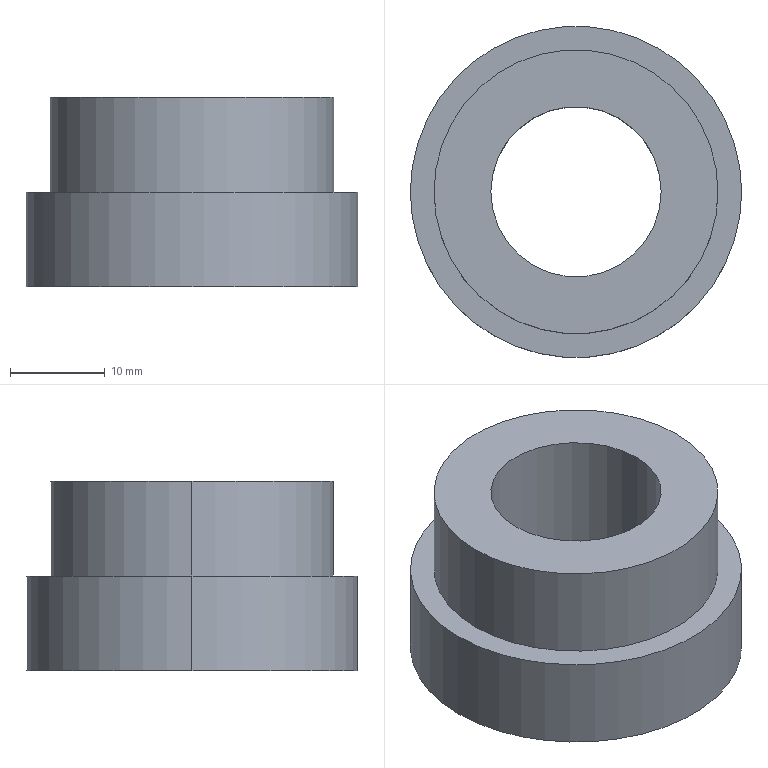Part | SolidWorks | features ICE 2, Extrusion 1 | 1 solid | 9 faces | box 35 x 35 x 20 mm | volume 11600 mm3 | cylinder 6 | plane 3 | commonest cylinder face diameters 18 x2 30 x2 35 x2
STEP:
#1=CARTESIAN_POINT('',(-9.,0.,0.));
#2=VERTEX_POINT('',#1);
#3=CARTESIAN_POINT('',(9.,0.,0.));
#4=VERTEX_POINT('',#3);
#5=CARTESIAN_POINT('',(0.,0.,0.));
#6=DIRECTION('',(0.,0.,1.));
#7=DIRECTION('',(1.,0.,0.));
#8=AXIS2_PLACEMENT_3D('',#5,#6,#7);
#9=CIRCLE('',#8,9.);
#10=EDGE_CURVE('',#2,#4,#9,.T.);
#11=ORIENTED_EDGE('',*,*,#10,.F.);
#12=CARTESIAN_POINT('',(-9.,0.,20.));
#13=VERTEX_POINT('',#12);
#14=CARTESIAN_POINT('',(-9.,0.,0.));
#15=DIRECTION('',(0.,0.,1.));
#16=VECTOR('',#15,1000.);
#17=LINE('',#14,#16);
#18=EDGE_CURVE('',#2,#13,#17,.T.);
#19=ORIENTED_EDGE('',*,*,#18,.T.);
#20=CARTESIAN_POINT('',(9.,0.,20.));
#21=VERTEX_POINT('',#20);
#22=CARTESIAN_POINT('',(0.,0.,20.));
#23=DIRECTION('',(0.,0.,1.));
#24=DIRECTION('',(1.,0.,0.));
#25=AXIS2_PLACEMENT_3D('',#22,#23,#24);
#26=CIRCLE('',#25,9.);
#27=EDGE_CURVE('',#13,#21,#26,.T.);
#28=ORIENTED_EDGE('',*,*,#27,.T.);
#29=CARTESIAN_POINT('',(9.,0.,0.));
#30=DIRECTION('',(0.,0.,1.));
#31=VECTOR('',#30,1000.);
#32=LINE('',#29,#31);
#33=EDGE_CURVE('',#4,#21,#32,.T.);
#34=ORIENTED_EDGE('',*,*,#33,.F.);
#35=EDGE_LOOP('',(#11,#19,#28,#34));
#36=FACE_OUTER_BOUND('',#35,.T.);
#37=CARTESIAN_POINT('',(0.,0.,0.));
#38=DIRECTION('',(0.,0.,1.));
#39=DIRECTION('',(1.,0.,0.));
#40=AXIS2_PLACEMENT_3D('',#37,#38,#39);
#41=CYLINDRICAL_SURFACE('',#40,9.);
#42=ADVANCED_FACE('',(#36),#41,.F.);
#43=CARTESIAN_POINT('',(15.,0.,20.));
#44=VERTEX_POINT('',#43);
#45=CARTESIAN_POINT('',(-15.,0.,20.));
#46=VERTEX_POINT('',#45);
#47=CARTESIAN_POINT('',(0.,0.,20.));
#48=DIRECTION('',(0.,0.,1.));
#49=DIRECTION('',(1.,0.,0.));
#50=AXIS2_PLACEMENT_3D('',#47,#48,#49);
#51=CIRCLE('',#50,15.);
#52=EDGE_CURVE('',#44,#46,#51,.T.);
#53=ORIENTED_EDGE('',*,*,#52,.F.);
#54=CARTESIAN_POINT('',(15.,0.,10.));
#55=VERTEX_POINT('',#54);
#56=CARTESIAN_POINT('',(15.,0.,20.));
#57=DIRECTION('',(0.,0.,-1.));
#58=VECTOR('',#57,1000.);
#59=LINE('',#56,#58);
#60=EDGE_CURVE('',#44,#55,#59,.T.);
#61=ORIENTED_EDGE('',*,*,#60,.T.);
#62=CARTESIAN_POINT('',(-15.,0.,10.));
#63=VERTEX_POINT('',#62);
#64=CARTESIAN_POINT('',(0.,0.,10.));
#65=DIRECTION('',(0.,0.,1.));
#66=DIRECTION('',(1.,0.,0.));
#67=AXIS2_PLACEMENT_3D('',#64,#65,#66);
#68=CIRCLE('',#67,15.);
#69=EDGE_CURVE('',#55,#63,#68,.T.);
#70=ORIENTED_EDGE('',*,*,#69,.T.);
#71=CARTESIAN_POINT('',(-15.,0.,20.));
#72=DIRECTION('',(0.,0.,-1.));
#73=VECTOR('',#72,1000.);
#74=LINE('',#71,#73);
#75=EDGE_CURVE('',#46,#63,#74,.T.);
#76=ORIENTED_EDGE('',*,*,#75,.F.);
#77=EDGE_LOOP('',(#53,#61,#70,#76));
#78=FACE_OUTER_BOUND('',#77,.T.);
#79=CARTESIAN_POINT('',(0.,0.,20.));
#80=DIRECTION('',(0.,0.,-1.));
#81=DIRECTION('',(-1.,0.,0.));
#82=AXIS2_PLACEMENT_3D('',#79,#80,#81);
#83=CYLINDRICAL_SURFACE('',#82,15.);
#84=ADVANCED_FACE('',(#78),#83,.T.);
#85=CARTESIAN_POINT('',(17.5,0.,10.));
#86=VERTEX_POINT('',#85);
#87=CARTESIAN_POINT('',(-17.5,0.,10.));
#88=VERTEX_POINT('',#87);
#89=CARTESIAN_POINT('',(0.,0.,10.));
#90=DIRECTION('',(0.,0.,1.));
#91=DIRECTION('',(1.,0.,0.));
#92=AXIS2_PLACEMENT_3D('',#89,#90,#91);
#93=CIRCLE('',#92,17.5);
#94=EDGE_CURVE('',#86,#88,#93,.T.);
#95=ORIENTED_EDGE('',*,*,#94,.F.);
#96=CARTESIAN_POINT('',(17.5,0.,0.));
#97=VERTEX_POINT('',#96);
#98=CARTESIAN_POINT('',(17.5,0.,10.));
#99=DIRECTION('',(0.,0.,-1.));
#100=VECTOR('',#99,1000.);
#101=LINE('',#98,#100);
#102=EDGE_CURVE('',#86,#97,#101,.T.);
#103=ORIENTED_EDGE('',*,*,#102,.T.);
#104=CARTESIAN_POINT('',(-17.5,0.,0.));
#105=VERTEX_POINT('',#104);
#106=CARTESIAN_POINT('',(0.,0.,0.));
#107=DIRECTION('',(0.,0.,1.));
#108=DIRECTION('',(1.,0.,0.));
#109=AXIS2_PLACEMENT_3D('',#106,#107,#108);
#110=CIRCLE('',#109,17.5);
#111=EDGE_CURVE('',#97,#105,#110,.T.);
#112=ORIENTED_EDGE('',*,*,#111,.T.);
#113=CARTESIAN_POINT('',(-17.5,0.,10.));
#114=DIRECTION('',(0.,0.,-1.));
#115=VECTOR('',#114,1000.);
#116=LINE('',#113,#115);
#117=EDGE_CURVE('',#88,#105,#116,.T.);
#118=ORIENTED_EDGE('',*,*,#117,.F.);
#119=EDGE_LOOP('',(#95,#103,#112,#118));
#120=FACE_OUTER_BOUND('',#119,.T.);
#121=CARTESIAN_POINT('',(0.,0.,10.));
#122=DIRECTION('',(0.,0.,-1.));
#123=DIRECTION('',(-1.,0.,0.));
#124=AXIS2_PLACEMENT_3D('',#121,#122,#123);
#125=CYLINDRICAL_SURFACE('',#124,17.5);
#126=ADVANCED_FACE('',(#120),#125,.T.);
#127=CARTESIAN_POINT('',(0.,0.,10.));
#128=DIRECTION('',(0.,0.,1.));
#129=DIRECTION('',(1.,0.,0.));
#130=AXIS2_PLACEMENT_3D('',#127,#128,#129);
#131=CIRCLE('',#130,17.5);
#132=EDGE_CURVE('',#88,#86,#131,.T.);
#133=ORIENTED_EDGE('',*,*,#132,.T.);
#134=ORIENTED_EDGE('',*,*,#94,.T.);
#135=EDGE_LOOP('',(#133,#134));
#136=FACE_OUTER_BOUND('',#135,.T.);
#137=CARTESIAN_POINT('',(0.,0.,10.));
#138=DIRECTION('',(0.,0.,1.));
#139=DIRECTION('',(1.,0.,0.));
#140=AXIS2_PLACEMENT_3D('',#137,#138,#139);
#141=CIRCLE('',#140,15.);
#142=EDGE_CURVE('',#63,#55,#141,.T.);
#143=ORIENTED_EDGE('',*,*,#142,.F.);
#144=ORIENTED_EDGE('',*,*,#69,.F.);
#145=EDGE_LOOP('',(#143,#144));
#146=FACE_BOUND('',#145,.T.);
#147=CARTESIAN_POINT('',(0.,0.,10.));
#148=DIRECTION('',(0.,0.,1.));
#149=DIRECTION('',(1.,0.,0.));
#150=AXIS2_PLACEMENT_3D('',#147,#148,#149);
#151=PLANE('',#150);
#152=ADVANCED_FACE('',(#136,#146),#151,.T.);
#153=ORIENTED_EDGE('',*,*,#102,.F.);
#154=ORIENTED_EDGE('',*,*,#132,.F.);
#155=ORIENTED_EDGE('',*,*,#117,.T.);
#156=CARTESIAN_POINT('',(0.,0.,0.));
#157=DIRECTION('',(0.,0.,1.));
#158=DIRECTION('',(1.,0.,0.));
#159=AXIS2_PLACEMENT_3D('',#156,#157,#158);
#160=CIRCLE('',#159,17.5);
#161=EDGE_CURVE('',#105,#97,#160,.T.);
#162=ORIENTED_EDGE('',*,*,#161,.T.);
#163=EDGE_LOOP('',(#153,#154,#155,#162));
#164=FACE_OUTER_BOUND('',#163,.T.);
#165=CARTESIAN_POINT('',(0.,0.,10.));
#166=DIRECTION('',(0.,0.,-1.));
#167=DIRECTION('',(-1.,0.,0.));
#168=AXIS2_PLACEMENT_3D('',#165,#166,#167);
#169=CYLINDRICAL_SURFACE('',#168,17.5);
#170=ADVANCED_FACE('',(#164),#169,.T.);
#171=CARTESIAN_POINT('',(0.,0.,0.));
#172=DIRECTION('',(0.,0.,1.));
#173=DIRECTION('',(1.,0.,0.));
#174=AXIS2_PLACEMENT_3D('',#171,#172,#173);
#175=CIRCLE('',#174,9.);
#176=EDGE_CURVE('',#4,#2,#175,.T.);
#177=ORIENTED_EDGE('',*,*,#176,.T.);
#178=ORIENTED_EDGE('',*,*,#10,.T.);
#179=EDGE_LOOP('',(#177,#178));
#180=FACE_BOUND('',#179,.T.);
#181=ORIENTED_EDGE('',*,*,#161,.F.);
#182=ORIENTED_EDGE('',*,*,#111,.F.);
#183=EDGE_LOOP('',(#181,#182));
#184=FACE_OUTER_BOUND('',#183,.T.);
#185=CARTESIAN_POINT('',(0.,0.,0.));
#186=DIRECTION('',(0.,0.,1.));
#187=DIRECTION('',(1.,0.,0.));
#188=AXIS2_PLACEMENT_3D('',#185,#186,#187);
#189=PLANE('',#188);
#190=ADVANCED_FACE('',(#180,#184),#189,.F.);
#191=ORIENTED_EDGE('',*,*,#60,.F.);
#192=CARTESIAN_POINT('',(0.,0.,20.));
#193=DIRECTION('',(0.,0.,1.));
#194=DIRECTION('',(1.,0.,0.));
#195=AXIS2_PLACEMENT_3D('',#192,#193,#194);
#196=CIRCLE('',#195,15.);
#197=EDGE_CURVE('',#46,#44,#196,.T.);
#198=ORIENTED_EDGE('',*,*,#197,.F.);
#199=ORIENTED_EDGE('',*,*,#75,.T.);
#200=ORIENTED_EDGE('',*,*,#142,.T.);
#201=EDGE_LOOP('',(#191,#198,#199,#200));
#202=FACE_OUTER_BOUND('',#201,.T.);
#203=CARTESIAN_POINT('',(0.,0.,20.));
#204=DIRECTION('',(0.,0.,-1.));
#205=DIRECTION('',(-1.,0.,0.));
#206=AXIS2_PLACEMENT_3D('',#203,#204,#205);
#207=CYLINDRICAL_SURFACE('',#206,15.);
#208=ADVANCED_FACE('',(#202),#207,.T.);
#209=CARTESIAN_POINT('',(0.,0.,20.));
#210=DIRECTION('',(0.,0.,1.));
#211=DIRECTION('',(1.,0.,0.));
#212=AXIS2_PLACEMENT_3D('',#209,#210,#211);
#213=CIRCLE('',#212,9.);
#214=EDGE_CURVE('',#21,#13,#213,.T.);
#215=ORIENTED_EDGE('',*,*,#214,.F.);
#216=ORIENTED_EDGE('',*,*,#27,.F.);
#217=EDGE_LOOP('',(#215,#216));
#218=FACE_BOUND('',#217,.T.);
#219=ORIENTED_EDGE('',*,*,#197,.T.);
#220=ORIENTED_EDGE('',*,*,#52,.T.);
#221=EDGE_LOOP('',(#219,#220));
#222=FACE_OUTER_BOUND('',#221,.T.);
#223=CARTESIAN_POINT('',(0.,0.,20.));
#224=DIRECTION('',(0.,0.,1.));
#225=DIRECTION('',(1.,0.,0.));
#226=AXIS2_PLACEMENT_3D('',#223,#224,#225);
#227=PLANE('',#226);
#228=ADVANCED_FACE('',(#218,#222),#227,.T.);
#229=ORIENTED_EDGE('',*,*,#18,.F.);
#230=ORIENTED_EDGE('',*,*,#176,.F.);
#231=ORIENTED_EDGE('',*,*,#33,.T.);
#232=ORIENTED_EDGE('',*,*,#214,.T.);
#233=EDGE_LOOP('',(#229,#230,#231,#232));
#234=FACE_OUTER_BOUND('',#233,.T.);
#235=CARTESIAN_POINT('',(0.,0.,0.));
#236=DIRECTION('',(0.,0.,1.));
#237=DIRECTION('',(1.,0.,0.));
#238=AXIS2_PLACEMENT_3D('',#235,#236,#237);
#239=CYLINDRICAL_SURFACE('',#238,9.);
#240=ADVANCED_FACE('',(#234),#239,.F.);
#241=CLOSED_SHELL('',(#42,#84,#126,#152,#170,#190,#208,#228,#240));
#242=MANIFOLD_SOLID_BREP('',#241);
#243=CARTESIAN_POINT('',(0.,0.,0.));
#244=DIRECTION('',(0.,0.,1.));
#245=DIRECTION('',(1.,0.,0.));
#246=AXIS2_PLACEMENT_3D('',#243,#244,#245);
#247=(LENGTH_UNIT()NAMED_UNIT(*)SI_UNIT(.MILLI.,.METRE.));
#248=UNCERTAINTY_MEASURE_WITH_UNIT(LENGTH_MEASURE(0.00001),#247,'','');
#249=(NAMED_UNIT(*)PLANE_ANGLE_UNIT()SI_UNIT($,.RADIAN.));
#250=(NAMED_UNIT(*)SI_UNIT($,.STERADIAN.)SOLID_ANGLE_UNIT());
#251=(GEOMETRIC_REPRESENTATION_CONTEXT(3)GLOBAL_UNCERTAINTY_ASSIGNED_CONTEXT((#248))GLOBAL_UNIT_ASSIGNED_CONTEXT((#247,#249,#250))REPRESENTATION_CONTEXT('',''));
#252=ADVANCED_BREP_SHAPE_REPRESENTATION('',(#242,#246),#251);